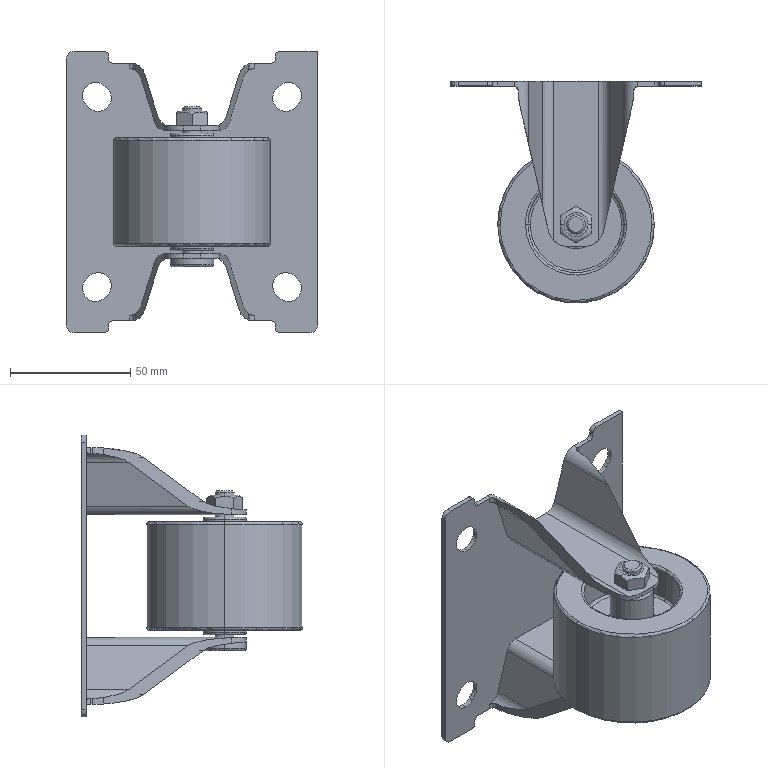Part | NX | features BREP 2 | 2 solids | 163 faces | box 104 x 92 x 117 mm | volume 154742 mm3 | cylinder 71 | plane 64 | torus 26 | cone 2 | commonest cylinder face diameters 4 x12 11 x12 12 x10 10 x8 40 x8 8 x6